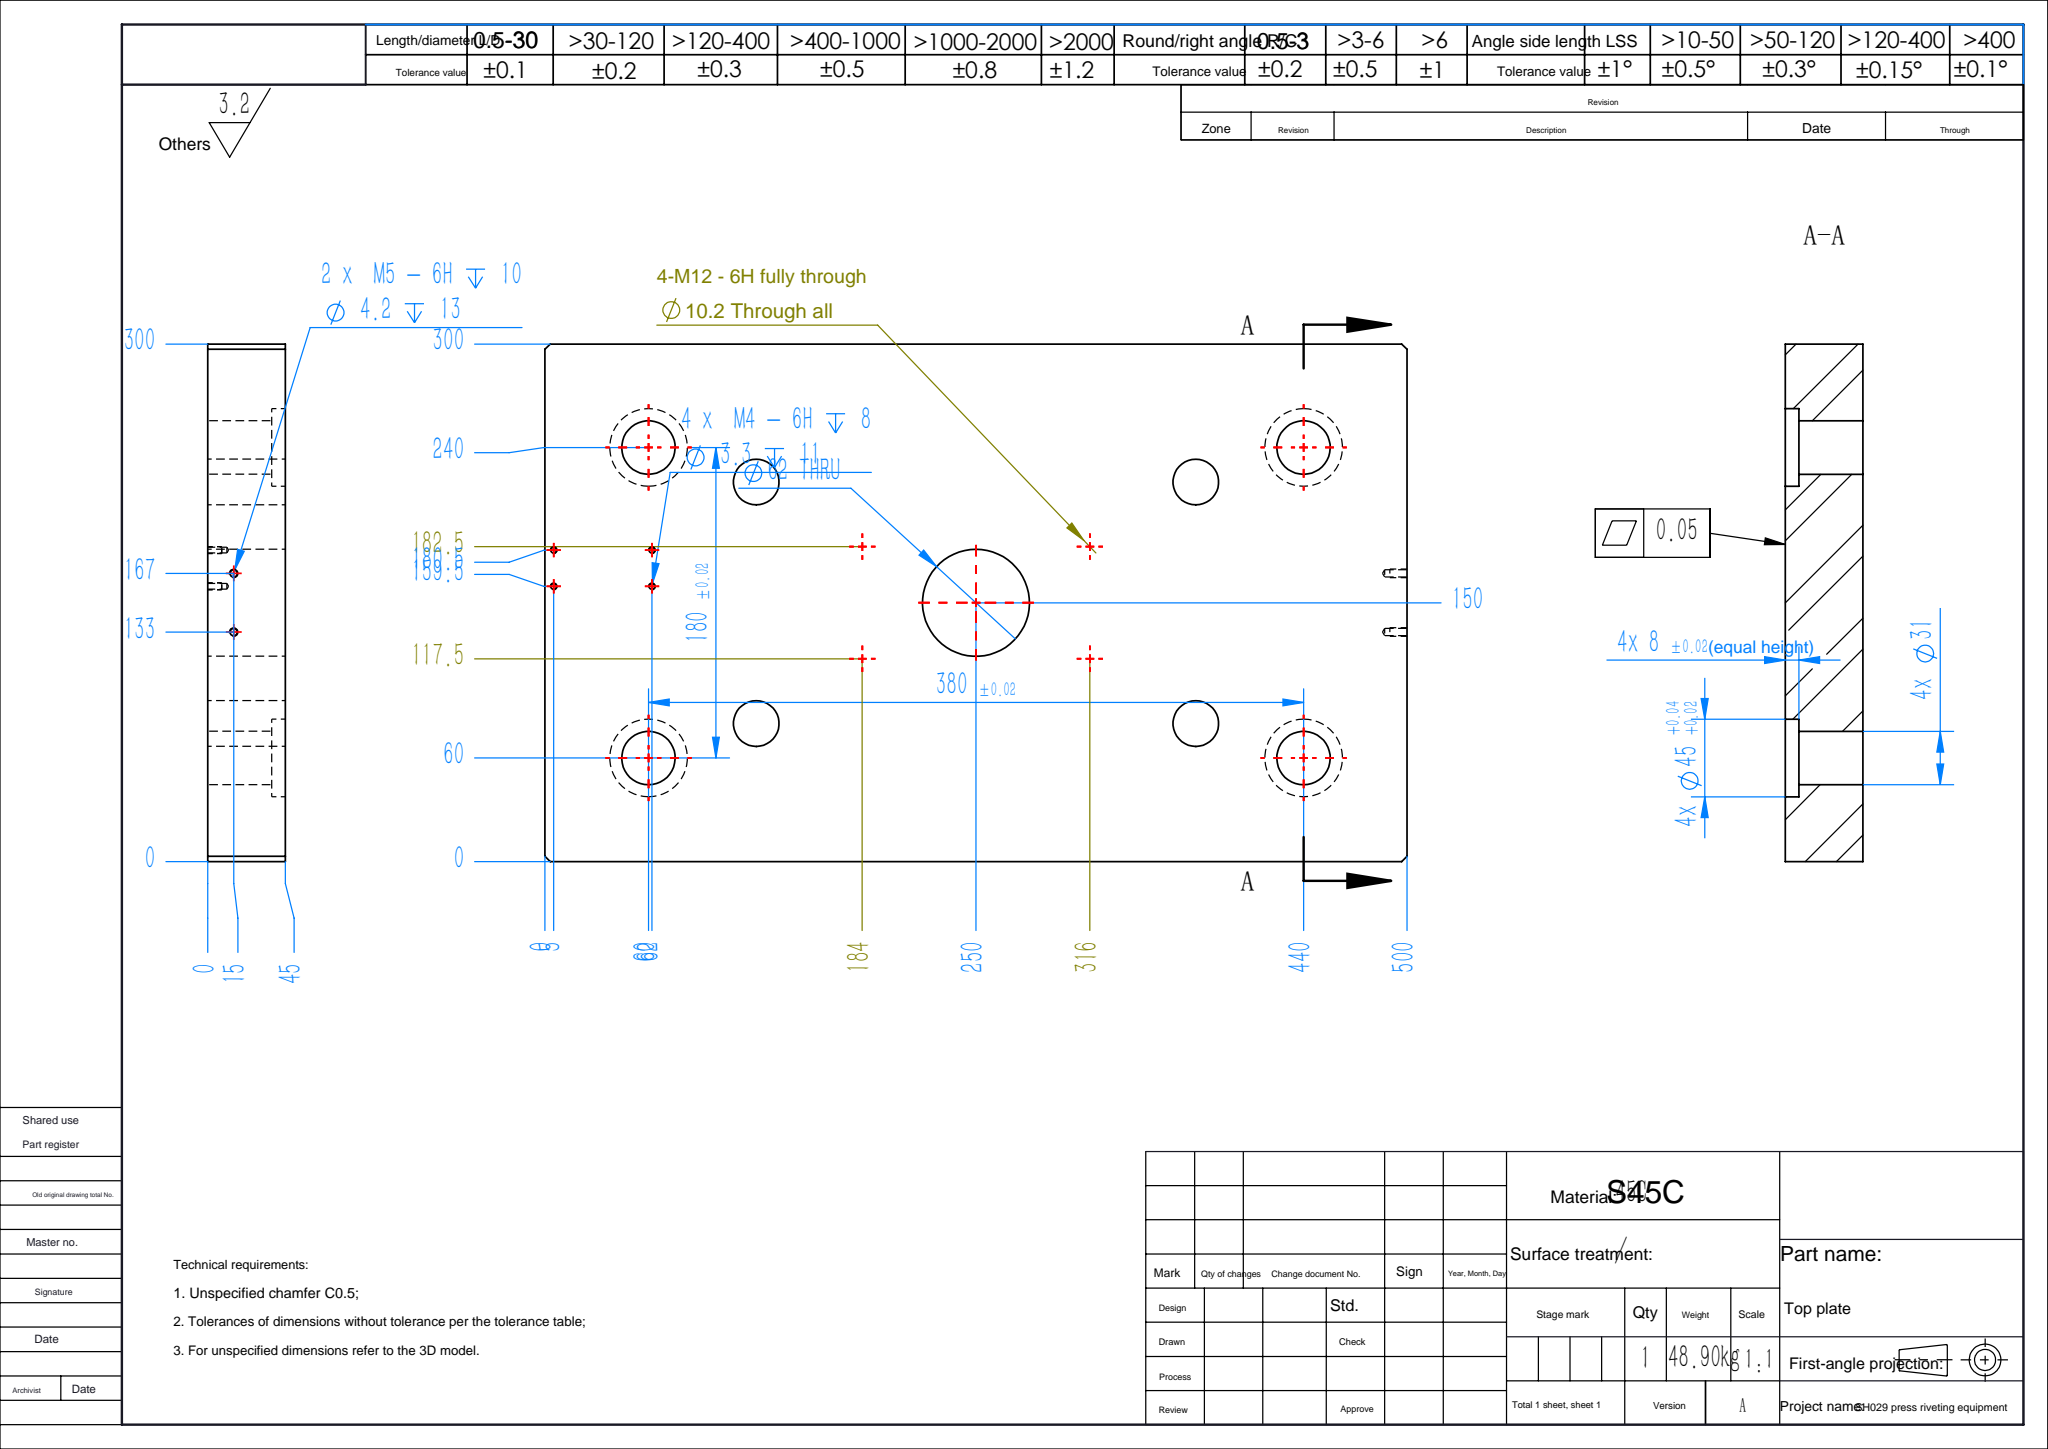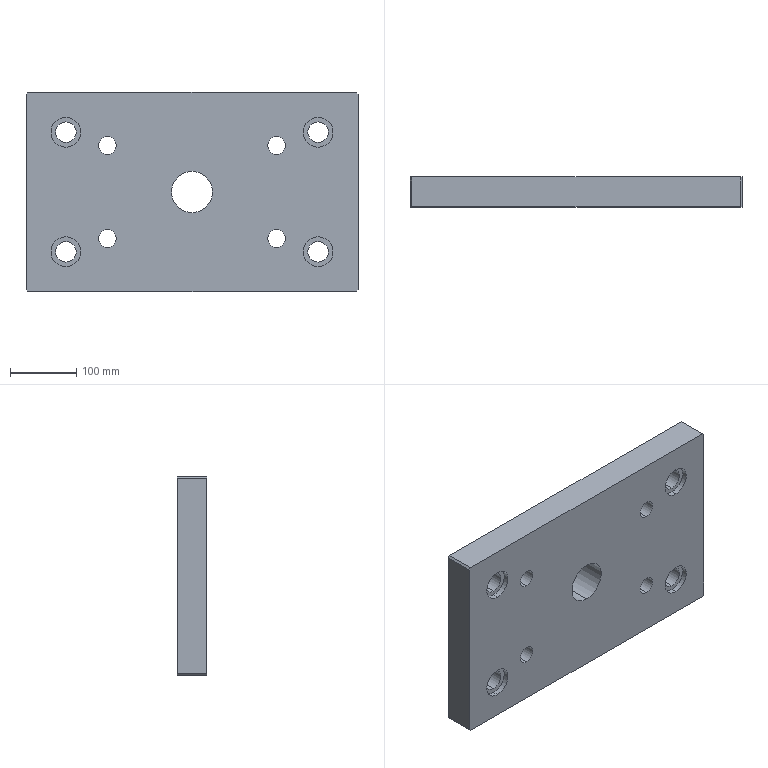Part | SolidWorks | features HoleWzd 3, ICE 2, Chamfer 1, Cut 1, Extrusion 1 | 1 solid | 64 faces | box 500 x 45 x 300 mm | volume 6350695 mm3 | cylinder 38 | plane 14 | cone 12 | commonest cylinder face diameters 3.3 x8 26.5 x8 31 x8 45 x8 4.2 x4 62 x2